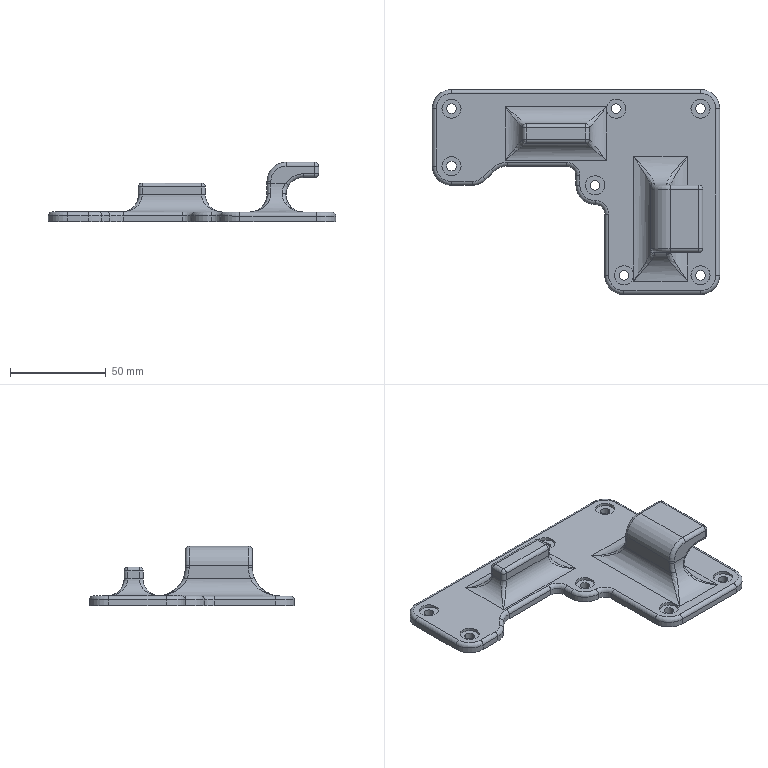Part | SolidWorks | features BaseBody 1 | 1 solid | 146 faces | box 150.006 x 107.003 x 31.143 mm | volume 74048 mm3 | cylinder 79 | plane 31 | torus 18 | spline 10 | sphere 8 | commonest cylinder face diameters 4 x29 10 x16 5 x14 20 x9 18 x7 6 x2